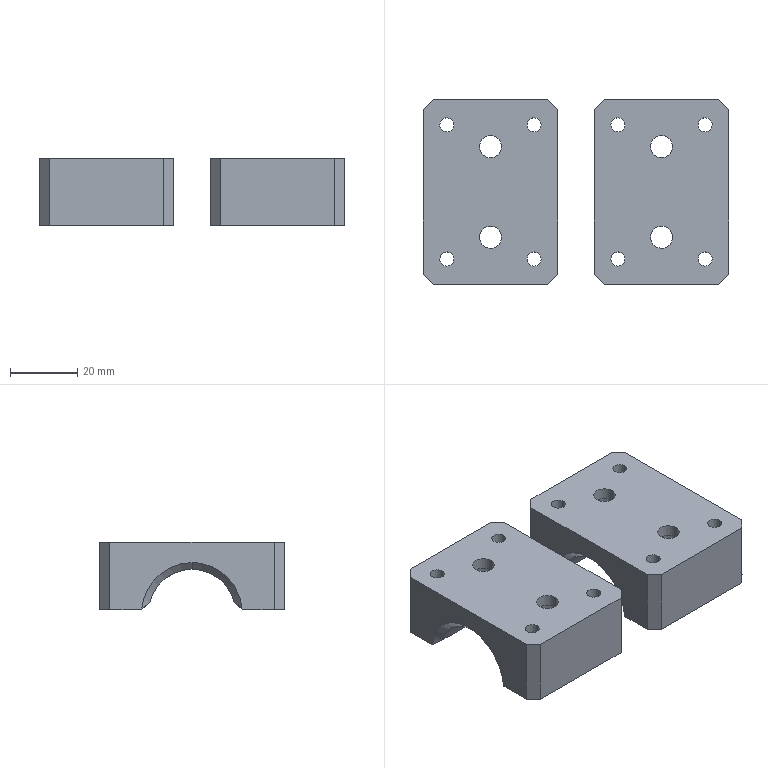NC program | NX | posted with a generic post | part box 91 x 55 x 20 mm
Lines 73 to 960 of 95737:
(ZLEVEL_PROFILE , TOOL : D10)
N126 T15 M6
N128 G54
N130 G17 G0 G90 X7.101 Y32.384 S9500 M3
N132 G43 Z30. H15
N134 Z1.5
N136 G94 G1 X7.946 Y32.6 Z1.454 F1000.
N138 X43.054 Z-0.386
N140 X44.463 Y32.24 Z-0.462
N142 X45.715 Y31.498 Z-0.538
N144 X49.498 Y27.715 Z-0.819
N146 X50.24 Y26.463 Z-0.895
N148 X50.6 Y25.054 Z-0.971
N150 Y24.5 Z-1.
N152 Y-24.5 F2800.
N154 G2 X49.106 Y-28.106 R5.1
N156 G1 X46.106 Y-31.106
N158 G2 X42.5 Y-32.6 R5.1
N160 G1 X8.5
N162 G2 X4.894 Y-31.106 R5.1
N164 G1 X1.894 Y-28.106
N166 G2 X0.4 Y-24.5 R5.1
N168 G1 Y24.5
N170 G2 X1.894 Y28.106 R5.1
N172 G1 X4.894 Y31.106
N174 G2 X8.5 Y32.6 R5.1
N176 G1 X42.5
N178 G2 X46.106 Y31.106 R5.1
N180 G1 X49.106 Y28.106
N182 G2 X50.6 Y24.5 R5.1
N184 G1 Y-24.274 Z-1.851
N186 X50.597 Y-24.661 Z-1.858
N188 X50.571 Y-25.047 Z-1.865
N190 X50.515 Y-25.43 Z-1.872
N192 X50.43 Y-25.808 Z-1.878
N194 X50.316 Y-26.178 Z-1.885
N196 X50.175 Y-26.538 Z-1.892
N198 X50.007 Y-26.887 Z-1.899
N200 X49.813 Y-27.221 Z-1.905
N202 X49.594 Y-27.541 Z-1.912
N204 X49.352 Y-27.842 Z-1.919
N206 X49.088 Y-28.125 Z-1.926
N208 X48.814 Y-28.399 Z-1.932
N210 X46.35 Y-30.862 Z-1.993
N212 X46.077 Y-31.136 Z-2.
N214 G2 X42.5 Y-32.6 R5.1
N216 G1 X8.5
N218 G2 X4.894 Y-31.106 R5.1
N220 G1 X1.894 Y-28.106
N222 G2 X0.4 Y-24.5 R5.1
N224 G1 Y24.5
N226 G2 X1.894 Y28.106 R5.1
N228 G1 X4.894 Y31.106
N230 G2 X8.5 Y32.6 R5.1
N232 G1 X42.5
N234 G2 X46.106 Y31.106 R5.1
N236 G1 X49.106 Y28.106
N238 G2 X50.6 Y24.5 R5.1
N240 G1 Y-24.274 Z-2.851
N242 X50.597 Y-24.661 Z-2.858
N244 X50.571 Y-25.047 Z-2.865
N246 X50.515 Y-25.43 Z-2.872
N248 X50.43 Y-25.808 Z-2.878
N250 X50.316 Y-26.178 Z-2.885
N252 X50.175 Y-26.538 Z-2.892
N254 X50.007 Y-26.887 Z-2.899
N256 X49.813 Y-27.221 Z-2.905
N258 X49.594 Y-27.541 Z-2.912
N260 X49.352 Y-27.842 Z-2.919
N262 X49.088 Y-28.125 Z-2.926
N264 X48.814 Y-28.399 Z-2.932
N266 X46.35 Y-30.862 Z-2.993
N268 X46.077 Y-31.136 Z-3.
N270 G2 X42.5 Y-32.6 R5.1
N272 G1 X8.5
N274 G2 X4.894 Y-31.106 R5.1
N276 G1 X1.894 Y-28.106
N278 G2 X0.4 Y-24.5 R5.1
N280 G1 Y24.5
N282 G2 X1.894 Y28.106 R5.1
N284 G1 X4.894 Y31.106
N286 G2 X8.5 Y32.6 R5.1
N288 G1 X42.5
N290 G2 X46.106 Y31.106 R5.1
N292 G1 X49.106 Y28.106
N294 G2 X50.6 Y24.5 R5.1
N296 G1 Y-24.274 Z-3.851
N298 X50.597 Y-24.661 Z-3.858
N300 X50.571 Y-25.047 Z-3.865
N302 X50.515 Y-25.43 Z-3.872
N304 X50.43 Y-25.808 Z-3.878
N306 X50.316 Y-26.178 Z-3.885
N308 X50.175 Y-26.538 Z-3.892
N310 X50.007 Y-26.887 Z-3.899
N312 X49.813 Y-27.221 Z-3.905
N314 X49.594 Y-27.541 Z-3.912
N316 X49.352 Y-27.842 Z-3.919
N318 X49.088 Y-28.125 Z-3.926
N320 X48.814 Y-28.399 Z-3.932
N322 X46.35 Y-30.862 Z-3.993
N324 X46.077 Y-31.136 Z-4.
N326 G2 X42.5 Y-32.6 R5.1
N328 G1 X8.5
N330 G2 X4.894 Y-31.106 R5.1
N332 G1 X1.894 Y-28.106
N334 G2 X0.4 Y-24.5 R5.1
N336 G1 Y24.5
N338 G2 X1.894 Y28.106 R5.1
N340 G1 X4.894 Y31.106
N342 G2 X8.5 Y32.6 R5.1
N344 G1 X42.5
N346 G2 X46.106 Y31.106 R5.1
N348 G1 X49.106 Y28.106
N350 G2 X50.6 Y24.5 R5.1
N352 G1 Y-24.274 Z-4.851
N354 X50.597 Y-24.661 Z-4.858
N356 X50.571 Y-25.047 Z-4.865
N358 X50.515 Y-25.43 Z-4.872
N360 X50.43 Y-25.808 Z-4.878
N362 X50.316 Y-26.178 Z-4.885
N364 X50.175 Y-26.538 Z-4.892
N366 X50.007 Y-26.887 Z-4.899
N368 X49.813 Y-27.221 Z-4.905
N370 X49.594 Y-27.541 Z-4.912
N372 X49.352 Y-27.842 Z-4.919
N374 X49.088 Y-28.125 Z-4.926
N376 X48.814 Y-28.399 Z-4.932
N378 X46.35 Y-30.862 Z-4.993
N380 X46.077 Y-31.136 Z-5.
N382 G2 X42.5 Y-32.6 R5.1
N384 G1 X8.5
N386 G2 X4.894 Y-31.106 R5.1
N388 G1 X1.894 Y-28.106
N390 G2 X0.4 Y-24.5 R5.1
N392 G1 Y24.5
N394 G2 X1.894 Y28.106 R5.1
N396 G1 X4.894 Y31.106
N398 G2 X8.5 Y32.6 R5.1
N400 G1 X42.5
N402 G2 X46.106 Y31.106 R5.1
N404 G1 X49.106 Y28.106
N406 G2 X50.6 Y24.5 R5.1
N408 G1 Y-24.274 Z-5.851
N410 X50.597 Y-24.661 Z-5.858
N412 X50.571 Y-25.047 Z-5.865
N414 X50.515 Y-25.43 Z-5.872
N416 X50.43 Y-25.808 Z-5.878
N418 X50.316 Y-26.178 Z-5.885
N420 X50.175 Y-26.538 Z-5.892
N422 X50.007 Y-26.887 Z-5.899
N424 X49.813 Y-27.221 Z-5.905
N426 X49.594 Y-27.541 Z-5.912
N428 X49.352 Y-27.842 Z-5.919
N430 X49.088 Y-28.125 Z-5.926
N432 X48.814 Y-28.399 Z-5.932
N434 X46.35 Y-30.862 Z-5.993
N436 X46.077 Y-31.136 Z-6.
N438 G2 X42.5 Y-32.6 R5.1
N440 G1 X8.5
N442 G2 X4.894 Y-31.106 R5.1
N444 G1 X1.894 Y-28.106
N446 G2 X0.4 Y-24.5 R5.1
N448 G1 Y24.5
N450 G2 X1.894 Y28.106 R5.1
N452 G1 X4.894 Y31.106
N454 G2 X8.5 Y32.6 R5.1
N456 G1 X42.5
N458 G2 X46.106 Y31.106 R5.1
N460 G1 X49.106 Y28.106
N462 G2 X50.6 Y24.5 R5.1
N464 G1 Y-24.274 Z-6.851
N466 X50.597 Y-24.661 Z-6.858
N468 X50.571 Y-25.047 Z-6.865
N470 X50.515 Y-25.43 Z-6.872
N472 X50.43 Y-25.808 Z-6.878
N474 X50.316 Y-26.178 Z-6.885
N476 X50.175 Y-26.538 Z-6.892
N478 X50.007 Y-26.887 Z-6.899
N480 X49.813 Y-27.221 Z-6.905
N482 X49.594 Y-27.541 Z-6.912
N484 X49.352 Y-27.842 Z-6.919
N486 X49.088 Y-28.125 Z-6.926
N488 X48.814 Y-28.399 Z-6.932
N490 X46.35 Y-30.862 Z-6.993
N492 X46.077 Y-31.136 Z-7.
N494 G2 X42.5 Y-32.6 R5.1
N496 G1 X8.5
N498 G2 X4.894 Y-31.106 R5.1
N500 G1 X1.894 Y-28.106
N502 G2 X0.4 Y-24.5 R5.1
N504 G1 Y24.5
N506 G2 X1.894 Y28.106 R5.1
N508 G1 X4.894 Y31.106
N510 G2 X8.5 Y32.6 R5.1
N512 G1 X42.5
N514 G2 X46.106 Y31.106 R5.1
N516 G1 X49.106 Y28.106
N518 G2 X50.6 Y24.5 R5.1
N520 G1 Y-24.274 Z-7.851
N522 X50.597 Y-24.661 Z-7.858
N524 X50.571 Y-25.047 Z-7.865
N526 X50.515 Y-25.43 Z-7.872
N528 X50.43 Y-25.808 Z-7.878
N530 X50.316 Y-26.178 Z-7.885
N532 X50.175 Y-26.538 Z-7.892
N534 X50.007 Y-26.887 Z-7.899
N536 X49.813 Y-27.221 Z-7.905
N538 X49.594 Y-27.541 Z-7.912
N540 X49.352 Y-27.842 Z-7.919
N542 X49.088 Y-28.125 Z-7.926
N544 X48.814 Y-28.399 Z-7.932
N546 X46.35 Y-30.862 Z-7.993
N548 X46.077 Y-31.136 Z-8.
N550 G2 X42.5 Y-32.6 R5.1
N552 G1 X8.5
N554 G2 X4.894 Y-31.106 R5.1
N556 G1 X1.894 Y-28.106
N558 G2 X0.4 Y-24.5 R5.1
N560 G1 Y24.5
N562 G2 X1.894 Y28.106 R5.1
N564 G1 X4.894 Y31.106
N566 G2 X8.5 Y32.6 R5.1
N568 G1 X42.5
N570 G2 X46.106 Y31.106 R5.1
N572 G1 X49.106 Y28.106
N574 G2 X50.6 Y24.5 R5.1
N576 G1 Y-24.274 Z-8.851
N578 X50.597 Y-24.661 Z-8.858
N580 X50.571 Y-25.047 Z-8.865
N582 X50.515 Y-25.43 Z-8.872
N584 X50.43 Y-25.808 Z-8.878
N586 X50.316 Y-26.178 Z-8.885
N588 X50.175 Y-26.538 Z-8.892
N590 X50.007 Y-26.887 Z-8.899
N592 X49.813 Y-27.221 Z-8.905
N594 X49.594 Y-27.541 Z-8.912
N596 X49.352 Y-27.842 Z-8.919
N598 X49.088 Y-28.125 Z-8.926
N600 X48.814 Y-28.399 Z-8.932
N602 X46.35 Y-30.862 Z-8.993
N604 X46.077 Y-31.136 Z-9.
N606 G2 X42.5 Y-32.6 R5.1
N608 G1 X8.5
N610 G2 X4.894 Y-31.106 R5.1
N612 G1 X1.894 Y-28.106
N614 G2 X0.4 Y-24.5 R5.1
N616 G1 Y24.5
N618 G2 X1.894 Y28.106 R5.1
N620 G1 X4.894 Y31.106
N622 G2 X8.5 Y32.6 R5.1
N624 G1 X42.5
N626 G2 X46.106 Y31.106 R5.1
N628 G1 X49.106 Y28.106
N630 G2 X50.6 Y24.5 R5.1
N632 G1 Y-24.274 Z-9.851
N634 X50.597 Y-24.661 Z-9.858
N636 X50.571 Y-25.047 Z-9.865
N638 X50.515 Y-25.43 Z-9.872
N640 X50.43 Y-25.808 Z-9.878
N642 X50.316 Y-26.178 Z-9.885
N644 X50.175 Y-26.538 Z-9.892
N646 X50.007 Y-26.887 Z-9.899
N648 X49.813 Y-27.221 Z-9.905
N650 X49.594 Y-27.541 Z-9.912
N652 X49.352 Y-27.842 Z-9.919
N654 X49.088 Y-28.125 Z-9.926
N656 X48.814 Y-28.399 Z-9.932
N658 X46.35 Y-30.862 Z-9.993
N660 X46.077 Y-31.136 Z-10.
N662 G2 X42.5 Y-32.6 R5.1
N664 G1 X8.5
N666 G2 X4.894 Y-31.106 R5.1
N668 G1 X1.894 Y-28.106
N670 G2 X0.4 Y-24.5 R5.1
N672 G1 Y24.5
N674 G2 X1.894 Y28.106 R5.1
N676 G1 X4.894 Y31.106
N678 G2 X8.5 Y32.6 R5.1
N680 G1 X42.5
N682 G2 X46.106 Y31.106 R5.1
N684 G1 X49.106 Y28.106
N686 G2 X50.6 Y24.5 R5.1
N688 G1 Y-24.274 Z-10.851
N690 X50.597 Y-24.661 Z-10.858
N692 X50.571 Y-25.047 Z-10.865
N694 X50.515 Y-25.43 Z-10.872
N696 X50.43 Y-25.808 Z-10.878
N698 X50.316 Y-26.178 Z-10.885
N700 X50.175 Y-26.538 Z-10.892
N702 X50.007 Y-26.887 Z-10.899
N704 X49.813 Y-27.221 Z-10.905
N706 X49.594 Y-27.541 Z-10.912
N708 X49.352 Y-27.842 Z-10.919
N710 X49.088 Y-28.125 Z-10.926
N712 X48.814 Y-28.399 Z-10.932
N714 X46.35 Y-30.862 Z-10.993
N716 X46.077 Y-31.136 Z-11.
N718 G2 X42.5 Y-32.6 R5.1
N720 G1 X8.5
N722 G2 X4.894 Y-31.106 R5.1
N724 G1 X1.894 Y-28.106
N726 G2 X0.4 Y-24.5 R5.1
N728 G1 Y24.5
N730 G2 X1.894 Y28.106 R5.1
N732 G1 X4.894 Y31.106
N734 G2 X8.5 Y32.6 R5.1
N736 G1 X42.5
N738 G2 X46.106 Y31.106 R5.1
N740 G1 X49.106 Y28.106
N742 G2 X50.6 Y24.5 R5.1
N744 G1 Y-24.274 Z-11.851
N746 X50.597 Y-24.661 Z-11.858
N748 X50.571 Y-25.047 Z-11.865
N750 X50.515 Y-25.43 Z-11.872
N752 X50.43 Y-25.808 Z-11.878
N754 X50.316 Y-26.178 Z-11.885
N756 X50.175 Y-26.538 Z-11.892
N758 X50.007 Y-26.887 Z-11.899
N760 X49.813 Y-27.221 Z-11.905
N762 X49.594 Y-27.541 Z-11.912
N764 X49.352 Y-27.842 Z-11.919
N766 X49.088 Y-28.125 Z-11.926
N768 X48.814 Y-28.399 Z-11.932
N770 X46.35 Y-30.862 Z-11.993
N772 X46.077 Y-31.136 Z-12.
N774 G2 X42.5 Y-32.6 R5.1
N776 G1 X8.5
N778 G2 X4.894 Y-31.106 R5.1
N780 G1 X1.894 Y-28.106
N782 G2 X0.4 Y-24.5 R5.1
N784 G1 Y24.5
N786 G2 X1.894 Y28.106 R5.1
N788 G1 X4.894 Y31.106
N790 G2 X8.5 Y32.6 R5.1
N792 G1 X42.5
N794 G2 X46.106 Y31.106 R5.1
N796 G1 X49.106 Y28.106
N798 G2 X50.6 Y24.5 R5.1
N800 G1 Y-24.274 Z-12.851
N802 X50.597 Y-24.661 Z-12.858
N804 X50.571 Y-25.047 Z-12.865
N806 X50.515 Y-25.43 Z-12.872
N808 X50.43 Y-25.808 Z-12.878
N810 X50.316 Y-26.178 Z-12.885
N812 X50.175 Y-26.538 Z-12.892
N814 X50.007 Y-26.887 Z-12.899
N816 X49.813 Y-27.221 Z-12.905
N818 X49.594 Y-27.541 Z-12.912
N820 X49.352 Y-27.842 Z-12.919
N822 X49.088 Y-28.125 Z-12.926
N824 X48.814 Y-28.399 Z-12.932
N826 X46.35 Y-30.862 Z-12.993
N828 X46.077 Y-31.136 Z-13.
N830 G2 X42.5 Y-32.6 R5.1
N832 G1 X8.5
N834 G2 X4.894 Y-31.106 R5.1
N836 G1 X1.894 Y-28.106
N838 G2 X0.4 Y-24.5 R5.1
N840 G1 Y24.5
N842 G2 X1.894 Y28.106 R5.1
N844 G1 X4.894 Y31.106
N846 G2 X8.5 Y32.6 R5.1
N848 G1 X42.5
N850 G2 X46.106 Y31.106 R5.1
N852 G1 X49.106 Y28.106
N854 G2 X50.6 Y24.5 R5.1
N856 G1 Y-24.274 Z-13.851
N858 X50.597 Y-24.661 Z-13.858
N860 X50.571 Y-25.047 Z-13.865
N862 X50.515 Y-25.43 Z-13.872
N864 X50.43 Y-25.808 Z-13.878
N866 X50.316 Y-26.178 Z-13.885
N868 X50.175 Y-26.538 Z-13.892
N870 X50.007 Y-26.887 Z-13.899
N872 X49.813 Y-27.221 Z-13.905
N874 X49.594 Y-27.541 Z-13.912
N876 X49.352 Y-27.842 Z-13.919
N878 X49.088 Y-28.125 Z-13.926
N880 X48.814 Y-28.399 Z-13.932
N882 X46.35 Y-30.862 Z-13.993
N884 X46.077 Y-31.136 Z-14.
N886 G2 X42.5 Y-32.6 R5.1
N888 G1 X8.5
N890 G2 X4.894 Y-31.106 R5.1
N892 G1 X1.894 Y-28.106
N894 G2 X0.4 Y-24.5 R5.1
N896 G1 Y24.5
N898 G2 X1.894 Y28.106 R5.1
N900 G1 X4.894 Y31.106
N902 G2 X8.5 Y32.6 R5.1
N904 G1 X42.5
N906 G2 X46.106 Y31.106 R5.1
N908 G1 X49.106 Y28.106
N910 G2 X50.6 Y24.5 R5.1
N912 G1 Y-24.274 Z-14.851
N914 X50.597 Y-24.661 Z-14.858
N916 X50.571 Y-25.047 Z-14.865
N918 X50.515 Y-25.43 Z-14.872
N920 X50.43 Y-25.808 Z-14.878
N922 X50.316 Y-26.178 Z-14.885
N924 X50.175 Y-26.538 Z-14.892
N926 X50.007 Y-26.887 Z-14.899
N928 X49.813 Y-27.221 Z-14.905
N930 X49.594 Y-27.541 Z-14.912
N932 X49.352 Y-27.842 Z-14.919
N934 X49.088 Y-28.125 Z-14.926
N936 X48.814 Y-28.399 Z-14.932
N938 X46.35 Y-30.862 Z-14.993
N940 X46.077 Y-31.136 Z-15.
N942 G2 X42.5 Y-32.6 R5.1
N944 G1 X8.5
N946 G2 X4.894 Y-31.106 R5.1
N948 G1 X1.894 Y-28.106
N950 G2 X0.4 Y-24.5 R5.1
N952 G1 Y24.5
N954 G2 X1.894 Y28.106 R5.1
N956 G1 X4.894 Y31.106
N958 G2 X8.5 Y32.6 R5.1
N960 G1 X42.5
N962 G2 X46.106 Y31.106 R5.1
N964 G1 X49.106 Y28.106
N966 G2 X50.6 Y24.5 R5.1
N968 G1 Y-24.274 Z-15.851
N970 X50.597 Y-24.661 Z-15.858
N972 X50.571 Y-25.047 Z-15.865
N974 X50.515 Y-25.43 Z-15.872
N976 X50.43 Y-25.808 Z-15.878
N978 X50.316 Y-26.178 Z-15.885
N980 X50.175 Y-26.538 Z-15.892
N982 X50.007 Y-26.887 Z-15.899
N984 X49.813 Y-27.221 Z-15.905
N986 X49.594 Y-27.541 Z-15.912
N988 X49.352 Y-27.842 Z-15.919
N990 X49.088 Y-28.125 Z-15.926
N992 X48.814 Y-28.399 Z-15.932
N994 X46.35 Y-30.862 Z-15.993
N996 X46.077 Y-31.136 Z-16.
N998 G2 X42.5 Y-32.6 R5.1
N1000 G1 X8.5
N1002 G2 X4.894 Y-31.106 R5.1
N1004 G1 X1.894 Y-28.106
N1006 G2 X0.4 Y-24.5 R5.1
N1008 G1 Y24.5
N1010 G2 X1.894 Y28.106 R5.1
N1012 G1 X4.894 Y31.106
N1014 G2 X8.5 Y32.6 R5.1
N1016 G1 X42.5
N1018 G2 X46.106 Y31.106 R5.1
N1020 G1 X49.106 Y28.106
N1022 G2 X50.6 Y24.5 R5.1
N1024 G1 Y-24.274 Z-16.851
N1026 X50.597 Y-24.661 Z-16.858
N1028 X50.571 Y-25.047 Z-16.865
N1030 X50.515 Y-25.43 Z-16.872
N1032 X50.43 Y-25.808 Z-16.878
N1034 X50.316 Y-26.178 Z-16.885
N1036 X50.175 Y-26.538 Z-16.892
N1038 X50.007 Y-26.887 Z-16.899
N1040 X49.813 Y-27.221 Z-16.905
N1042 X49.594 Y-27.541 Z-16.912
N1044 X49.352 Y-27.842 Z-16.919
N1046 X49.088 Y-28.125 Z-16.926
N1048 X48.814 Y-28.399 Z-16.932
N1050 X46.35 Y-30.862 Z-16.993
N1052 X46.077 Y-31.136 Z-17.
N1054 G2 X42.5 Y-32.6 R5.1
N1056 G1 X8.5
N1058 G2 X4.894 Y-31.106 R5.1
N1060 G1 X1.894 Y-28.106
N1062 G2 X0.4 Y-24.5 R5.1
N1064 G1 Y24.5
N1066 G2 X1.894 Y28.106 R5.1
N1068 G1 X4.894 Y31.106
N1070 G2 X8.5 Y32.6 R5.1
N1072 G1 X42.5
N1074 G2 X46.106 Y31.106 R5.1
N1076 G1 X49.106 Y28.106
N1078 G2 X50.6 Y24.5 R5.1
N1080 G1 Y-24.274 Z-17.851
N1082 X50.597 Y-24.661 Z-17.858
N1084 X50.571 Y-25.047 Z-17.865
N1086 X50.515 Y-25.43 Z-17.872
N1088 X50.43 Y-25.808 Z-17.878
N1090 X50.316 Y-26.178 Z-17.885
N1092 X50.175 Y-26.538 Z-17.892
N1094 X50.007 Y-26.887 Z-17.899
N1096 X49.813 Y-27.221 Z-17.905
N1098 X49.594 Y-27.541 Z-17.912
N1100 X49.352 Y-27.842 Z-17.919
N1102 X49.088 Y-28.125 Z-17.926
N1104 X48.814 Y-28.399 Z-17.932
N1106 X46.35 Y-30.862 Z-17.993
N1108 X46.077 Y-31.136 Z-18.
N1110 G2 X42.5 Y-32.6 R5.1
N1112 G1 X8.5
N1114 G2 X4.894 Y-31.106 R5.1
N1116 G1 X1.894 Y-28.106
N1118 G2 X0.4 Y-24.5 R5.1
N1120 G1 Y24.5
N1122 G2 X1.894 Y28.106 R5.1
N1124 G1 X4.894 Y31.106
N1126 G2 X8.5 Y32.6 R5.1
N1128 G1 X42.5
N1130 G2 X46.106 Y31.106 R5.1
N1132 G1 X49.106 Y28.106
N1134 G2 X50.6 Y24.5 R5.1
N1136 G1 Y-24.274 Z-18.851
N1138 X50.597 Y-24.661 Z-18.858
N1140 X50.571 Y-25.047 Z-18.865
N1142 X50.515 Y-25.43 Z-18.872
N1144 X50.43 Y-25.808 Z-18.878
N1146 X50.316 Y-26.178 Z-18.885
N1148 X50.175 Y-26.538 Z-18.892
N1150 X50.007 Y-26.887 Z-18.899
N1152 X49.813 Y-27.221 Z-18.905
N1154 X49.594 Y-27.541 Z-18.912
N1156 X49.352 Y-27.842 Z-18.919
N1158 X49.088 Y-28.125 Z-18.926
N1160 X48.814 Y-28.399 Z-18.932
N1162 X46.35 Y-30.862 Z-18.993
N1164 X46.077 Y-31.136 Z-19.
N1166 G2 X42.5 Y-32.6 R5.1
N1168 G1 X8.5
N1170 G2 X4.894 Y-31.106 R5.1
N1172 G1 X1.894 Y-28.106
N1174 G2 X0.4 Y-24.5 R5.1
N1176 G1 Y24.5
N1178 G2 X1.894 Y28.106 R5.1
N1180 G1 X4.894 Y31.106
N1182 G2 X8.5 Y32.6 R5.1
N1184 G1 X42.5
N1186 G2 X46.106 Y31.106 R5.1
N1188 G1 X49.106 Y28.106
N1190 G2 X50.6 Y24.5 R5.1
N1192 G1 Y-24.274 Z-19.851
N1194 X50.597 Y-24.661 Z-19.858
N1196 X50.571 Y-25.047 Z-19.865
N1198 X50.515 Y-25.43 Z-19.872
N1200 X50.43 Y-25.808 Z-19.878
N1202 X50.316 Y-26.178 Z-19.885
N1204 X50.175 Y-26.538 Z-19.892
N1206 X50.007 Y-26.887 Z-19.899
N1208 X49.813 Y-27.221 Z-19.905
N1210 X49.594 Y-27.541 Z-19.912
N1212 X49.352 Y-27.842 Z-19.919
N1214 X49.088 Y-28.125 Z-19.926
N1216 X48.814 Y-28.399 Z-19.932
N1218 X46.35 Y-30.862 Z-19.993
N1220 X46.077 Y-31.136 Z-20.
N1222 G2 X42.5 Y-32.6 R5.1
N1224 G1 X8.5
N1226 G2 X4.894 Y-31.106 R5.1
N1228 G1 X1.894 Y-28.106
N1230 G2 X0.4 Y-24.5 R5.1
N1232 G1 Y24.5
N1234 G2 X1.894 Y28.106 R5.1
N1236 G1 X4.894 Y31.106
N1238 G2 X8.5 Y32.6 R5.1
N1240 G1 X42.5
N1242 G2 X46.106 Y31.106 R5.1
N1244 G1 X49.106 Y28.106
N1246 G2 X50.6 Y24.5 R5.1
N1248 G1 Y-24.5
N1250 G2 X49.106 Y-28.106 R5.1
N1252 G1 X46.077 Y-31.136
N1254 Z-18.5
N1256 G0 Z53.
N1258 X-7.101 Y-32.384
N1260 Z1.5
N1262 G1 X-7.946 Y-32.6 Z1.454 F1000.
N1264 X-43.054 Z-0.386
N1266 X-44.463 Y-32.24 Z-0.462
N1268 X-45.715 Y-31.498 Z-0.538
N1270 X-49.498 Y-27.715 Z-0.819
N1272 X-50.24 Y-26.463 Z-0.895
N1274 X-50.6 Y-25.054 Z-0.971
N1276 Y-24.5 Z-1.
N1278 Y24.5 F2800.
N1280 G2 X-49.106 Y28.106 R5.1
N1282 G1 X-46.106 Y31.106
N1284 G2 X-42.5 Y32.6 R5.1
N1286 G1 X-8.5
N1288 G2 X-4.894 Y31.106 R5.1
N1290 G1 X-1.894 Y28.106
N1292 G2 X-0.4 Y24.5 R5.1
N1294 G1 Y-24.5
N1296 G2 X-1.894 Y-28.106 R5.1
N1298 G1 X-4.894 Y-31.106
N1300 G2 X-8.5 Y-32.6 R5.1
N1302 G1 X-42.5
N1304 G2 X-46.106 Y-31.106 R5.1
N1306 G1 X-49.106 Y-28.106
N1308 G2 X-50.6 Y-24.5 R5.1
N1310 G1 Y24.274 Z-1.851
N1312 X-50.597 Y24.661 Z-1.858
N1314 X-50.571 Y25.047 Z-1.865
N1316 X-50.515 Y25.43 Z-1.872
N1318 X-50.43 Y25.808 Z-1.878
N1320 X-50.316 Y26.178 Z-1.885
N1322 X-50.175 Y26.538 Z-1.892
N1324 X-50.007 Y26.887 Z-1.899
N1326 X-49.813 Y27.221 Z-1.905
N1328 X-49.594 Y27.541 Z-1.912
N1330 X-49.352 Y27.842 Z-1.919
N1332 X-49.088 Y28.125 Z-1.926
N1334 X-48.814 Y28.399 Z-1.932
N1336 X-46.35 Y30.862 Z-1.993
N1338 X-46.077 Y31.136 Z-2.
N1340 G2 X-42.5 Y32.6 R5.1
N1342 G1 X-8.5
N1344 G2 X-4.894 Y31.106 R5.1
N1346 G1 X-1.894 Y28.106
N1348 G2 X-0.4 Y24.5 R5.1
N1350 G1 Y-24.5
N1352 G2 X-1.894 Y-28.106 R5.1
N1354 G1 X-4.894 Y-31.106
N1356 G2 X-8.5 Y-32.6 R5.1
N1358 G1 X-42.5
N1360 G2 X-46.106 Y-31.106 R5.1
N1362 G1 X-49.106 Y-28.106
N1364 G2 X-50.6 Y-24.5 R5.1
N1366 G1 Y24.274 Z-2.851
N1368 X-50.597 Y24.661 Z-2.858
N1370 X-50.571 Y25.047 Z-2.865
N1372 X-50.515 Y25.43 Z-2.872
N1374 X-50.43 Y25.808 Z-2.878
N1376 X-50.316 Y26.178 Z-2.885
N1378 X-50.175 Y26.538 Z-2.892
N1380 X-50.007 Y26.887 Z-2.899
N1382 X-49.813 Y27.221 Z-2.905
N1384 X-49.594 Y27.541 Z-2.912
N1386 X-49.352 Y27.842 Z-2.919
N1388 X-49.088 Y28.125 Z-2.926
N1390 X-48.814 Y28.399 Z-2.932
N1392 X-46.35 Y30.862 Z-2.993
N1394 X-46.077 Y31.136 Z-3.
N1396 G2 X-42.5 Y32.6 R5.1
N1398 G1 X-8.5
N1400 G2 X-4.894 Y31.106 R5.1
N1402 G1 X-1.894 Y28.106
N1404 G2 X-0.4 Y24.5 R5.1
N1406 G1 Y-24.5
N1408 G2 X-1.894 Y-28.106 R5.1
N1410 G1 X-4.894 Y-31.106
N1412 G2 X-8.5 Y-32.6 R5.1
N1414 G1 X-42.5
N1416 G2 X-46.106 Y-31.106 R5.1
N1418 G1 X-49.106 Y-28.106
N1420 G2 X-50.6 Y-24.5 R5.1
N1422 G1 Y24.274 Z-3.851
N1424 X-50.597 Y24.661 Z-3.858
N1426 X-50.571 Y25.047 Z-3.865
N1428 X-50.515 Y25.43 Z-3.872
N1430 X-50.43 Y25.808 Z-3.878
N1432 X-50.316 Y26.178 Z-3.885
N1434 X-50.175 Y26.538 Z-3.892
N1436 X-50.007 Y26.887 Z-3.899
N1438 X-49.813 Y27.221 Z-3.905
N1440 X-49.594 Y27.541 Z-3.912
N1442 X-49.352 Y27.842 Z-3.919
N1444 X-49.088 Y28.125 Z-3.926
N1446 X-48.814 Y28.399 Z-3.932
N1448 X-46.35 Y30.862 Z-3.993
N1450 X-46.077 Y31.136 Z-4.
N1452 G2 X-42.5 Y32.6 R5.1
N1454 G1 X-8.5
N1456 G2 X-4.894 Y31.106 R5.1
N1458 G1 X-1.894 Y28.106
N1460 G2 X-0.4 Y24.5 R5.1
N1462 G1 Y-24.5
N1464 G2 X-1.894 Y-28.106 R5.1
N1466 G1 X-4.894 Y-31.106
N1468 G2 X-8.5 Y-32.6 R5.1
N1470 G1 X-42.5
N1472 G2 X-46.106 Y-31.106 R5.1
N1474 G1 X-49.106 Y-28.106
N1476 G2 X-50.6 Y-24.5 R5.1
N1478 G1 Y24.274 Z-4.851
N1480 X-50.597 Y24.661 Z-4.858
N1482 X-50.571 Y25.047 Z-4.865
N1484 X-50.515 Y25.43 Z-4.872
N1486 X-50.43 Y25.808 Z-4.878
N1488 X-50.316 Y26.178 Z-4.885
N1490 X-50.175 Y26.538 Z-4.892
N1492 X-50.007 Y26.887 Z-4.899
N1494 X-49.813 Y27.221 Z-4.905
N1496 X-49.594 Y27.541 Z-4.912
N1498 X-49.352 Y27.842 Z-4.919
N1500 X-49.088 Y28.125 Z-4.926
N1502 X-48.814 Y28.399 Z-4.932
N1504 X-46.35 Y30.862 Z-4.993
N1506 X-46.077 Y31.136 Z-5.
N1508 G2 X-42.5 Y32.6 R5.1
N1510 G1 X-8.5
N1512 G2 X-4.894 Y31.106 R5.1
N1514 G1 X-1.894 Y28.106
N1516 G2 X-0.4 Y24.5 R5.1
N1518 G1 Y-24.5
N1520 G2 X-1.894 Y-28.106 R5.1
N1522 G1 X-4.894 Y-31.106
N1524 G2 X-8.5 Y-32.6 R5.1
N1526 G1 X-42.5
N1528 G2 X-46.106 Y-31.106 R5.1
N1530 G1 X-49.106 Y-28.106
N1532 G2 X-50.6 Y-24.5 R5.1
N1534 G1 Y24.274 Z-5.851
N1536 X-50.597 Y24.661 Z-5.858
N1538 X-50.571 Y25.047 Z-5.865
N1540 X-50.515 Y25.43 Z-5.872
N1542 X-50.43 Y25.808 Z-5.878
N1544 X-50.316 Y26.178 Z-5.885
N1546 X-50.175 Y26.538 Z-5.892
N1548 X-50.007 Y26.887 Z-5.899
N1550 X-49.813 Y27.221 Z-5.905
N1552 X-49.594 Y27.541 Z-5.912
N1554 X-49.352 Y27.842 Z-5.919
N1556 X-49.088 Y28.125 Z-5.926
N1558 X-48.814 Y28.399 Z-5.932
N1560 X-46.35 Y30.862 Z-5.993
N1562 X-46.077 Y31.136 Z-6.
N1564 G2 X-42.5 Y32.6 R5.1
N1566 G1 X-8.5
N1568 G2 X-4.894 Y31.106 R5.1
N1570 G1 X-1.894 Y28.106
N1572 G2 X-0.4 Y24.5 R5.1
N1574 G1 Y-24.5
N1576 G2 X-1.894 Y-28.106 R5.1
N1578 G1 X-4.894 Y-31.106
N1580 G2 X-8.5 Y-32.6 R5.1
N1582 G1 X-42.5
N1584 G2 X-46.106 Y-31.106 R5.1
N1586 G1 X-49.106 Y-28.106
N1588 G2 X-50.6 Y-24.5 R5.1
N1590 G1 Y24.274 Z-6.851
N1592 X-50.597 Y24.661 Z-6.858
N1594 X-50.571 Y25.047 Z-6.865
N1596 X-50.515 Y25.43 Z-6.872
N1598 X-50.43 Y25.808 Z-6.878
N1600 X-50.316 Y26.178 Z-6.885
N1602 X-50.175 Y26.538 Z-6.892
N1604 X-50.007 Y26.887 Z-6.899
N1606 X-49.813 Y27.221 Z-6.905
N1608 X-49.594 Y27.541 Z-6.912
N1610 X-49.352 Y27.842 Z-6.919
N1612 X-49.088 Y28.125 Z-6.926
N1614 X-48.814 Y28.399 Z-6.932
N1616 X-46.35 Y30.862 Z-6.993
N1618 X-46.077 Y31.136 Z-7.
N1620 G2 X-42.5 Y32.6 R5.1
N1622 G1 X-8.5
N1624 G2 X-4.894 Y31.106 R5.1
N1626 G1 X-1.894 Y28.106
N1628 G2 X-0.4 Y24.5 R5.1
N1630 G1 Y-24.5
N1632 G2 X-1.894 Y-28.106 R5.1
N1634 G1 X-4.894 Y-31.106
N1636 G2 X-8.5 Y-32.6 R5.1
N1638 G1 X-42.5
N1640 G2 X-46.106 Y-31.106 R5.1
N1642 G1 X-49.106 Y-28.106
N1644 G2 X-50.6 Y-24.5 R5.1
N1646 G1 Y24.274 Z-7.851
N1648 X-50.597 Y24.661 Z-7.858
N1650 X-50.571 Y25.047 Z-7.865
N1652 X-50.515 Y25.43 Z-7.872
N1654 X-50.43 Y25.808 Z-7.878
N1656 X-50.316 Y26.178 Z-7.885
N1658 X-50.175 Y26.538 Z-7.892
N1660 X-50.007 Y26.887 Z-7.899
N1662 X-49.813 Y27.221 Z-7.905
N1664 X-49.594 Y27.541 Z-7.912
N1666 X-49.352 Y27.842 Z-7.919
N1668 X-49.088 Y28.125 Z-7.926
N1670 X-48.814 Y28.399 Z-7.932
N1672 X-46.35 Y30.862 Z-7.993
N1674 X-46.077 Y31.136 Z-8.
N1676 G2 X-42.5 Y32.6 R5.1
N1678 G1 X-8.5
N1680 G2 X-4.894 Y31.106 R5.1
N1682 G1 X-1.894 Y28.106
N1684 G2 X-0.4 Y24.5 R5.1
N1686 G1 Y-24.5
N1688 G2 X-1.894 Y-28.106 R5.1
N1690 G1 X-4.894 Y-31.106
N1692 G2 X-8.5 Y-32.6 R5.1
N1694 G1 X-42.5
N1696 G2 X-46.106 Y-31.106 R5.1
N1698 G1 X-49.106 Y-28.106
N1700 G2 X-50.6 Y-24.5 R5.1
N1702 G1 Y24.274 Z-8.851
N1704 X-50.597 Y24.661 Z-8.858
N1706 X-50.571 Y25.047 Z-8.865
N1708 X-50.515 Y25.43 Z-8.872
N1710 X-50.43 Y25.808 Z-8.878
N1712 X-50.316 Y26.178 Z-8.885
N1714 X-50.175 Y26.538 Z-8.892
N1716 X-50.007 Y26.887 Z-8.899
N1718 X-49.813 Y27.221 Z-8.905
N1720 X-49.594 Y27.541 Z-8.912
N1722 X-49.352 Y27.842 Z-8.919
N1724 X-49.088 Y28.125 Z-8.926
N1726 X-48.814 Y28.399 Z-8.932
N1728 X-46.35 Y30.862 Z-8.993
N1730 X-46.077 Y31.136 Z-9.
N1732 G2 X-42.5 Y32.6 R5.1
N1734 G1 X-8.5
N1736 G2 X-4.894 Y31.106 R5.1
N1738 G1 X-1.894 Y28.106
N1740 G2 X-0.4 Y24.5 R5.1
N1742 G1 Y-24.5
N1744 G2 X-1.894 Y-28.106 R5.1
N1746 G1 X-4.894 Y-31.106
N1748 G2 X-8.5 Y-32.6 R5.1
N1750 G1 X-42.5
N1752 G2 X-46.106 Y-31.106 R5.1
N1754 G1 X-49.106 Y-28.106
N1756 G2 X-50.6 Y-24.5 R5.1
N1758 G1 Y24.274 Z-9.851
N1760 X-50.597 Y24.661 Z-9.858
N1762 X-50.571 Y25.047 Z-9.865
N1764 X-50.515 Y25.43 Z-9.872
N1766 X-50.43 Y25.808 Z-9.878
N1768 X-50.316 Y26.178 Z-9.885
N1770 X-50.175 Y26.538 Z-9.892
N1772 X-50.007 Y26.887 Z-9.899
N1774 X-49.813 Y27.221 Z-9.905
N1776 X-49.594 Y27.541 Z-9.912
N1778 X-49.352 Y27.842 Z-9.919
N1780 X-49.088 Y28.125 Z-9.926
N1782 X-48.814 Y28.399 Z-9.932
N1784 X-46.35 Y30.862 Z-9.993
N1786 X-46.077 Y31.136 Z-10.
N1788 G2 X-42.5 Y32.6 R5.1
N1790 G1 X-8.5
N1792 G2 X-4.894 Y31.106 R5.1
N1794 G1 X-1.894 Y28.106
N1796 G2 X-0.4 Y24.5 R5.1
N1798 G1 Y-24.5
N1800 G2 X-1.894 Y-28.106 R5.1
N1802 G1 X-4.894 Y-31.106
N1804 G2 X-8.5 Y-32.6 R5.1
N1806 G1 X-42.5
N1808 G2 X-46.106 Y-31.106 R5.1
N1810 G1 X-49.106 Y-28.106
N1812 G2 X-50.6 Y-24.5 R5.1
N1814 G1 Y24.274 Z-10.851
N1816 X-50.597 Y24.661 Z-10.858
N1818 X-50.571 Y25.047 Z-10.865
N1820 X-50.515 Y25.43 Z-10.872
N1822 X-50.43 Y25.808 Z-10.878
N1824 X-50.316 Y26.178 Z-10.885
N1826 X-50.175 Y26.538 Z-10.892
N1828 X-50.007 Y26.887 Z-10.899
N1830 X-49.813 Y27.221 Z-10.905
N1832 X-49.594 Y27.541 Z-10.912
N1834 X-49.352 Y27.842 Z-10.919
N1836 X-49.088 Y28.125 Z-10.926
N1838 X-48.814 Y28.399 Z-10.932
N1840 X-46.35 Y30.862 Z-10.993
N1842 X-46.077 Y31.136 Z-11.
N1844 G2 X-42.5 Y32.6 R5.1
N1846 G1 X-8.5
N1848 G2 X-4.894 Y31.106 R5.1
N1850 G1 X-1.894 Y28.106
N1852 G2 X-0.4 Y24.5 R5.1
N1854 G1 Y-24.5
N1856 G2 X-1.894 Y-28.106 R5.1
N1858 G1 X-4.894 Y-31.106
N1860 G2 X-8.5 Y-32.6 R5.1
N1862 G1 X-42.5
N1864 G2 X-46.106 Y-31.106 R5.1
N1866 G1 X-49.106 Y-28.106
N1868 G2 X-50.6 Y-24.5 R5.1
N1870 G1 Y24.274 Z-11.851
N1872 X-50.597 Y24.661 Z-11.858
N1874 X-50.571 Y25.047 Z-11.865
N1876 X-50.515 Y25.43 Z-11.872
N1878 X-50.43 Y25.808 Z-11.878
N1880 X-50.316 Y26.178 Z-11.885
N1882 X-50.175 Y26.538 Z-11.892
N1884 X-50.007 Y26.887 Z-11.899
N1886 X-49.813 Y27.221 Z-11.905
N1888 X-49.594 Y27.541 Z-11.912
N1890 X-49.352 Y27.842 Z-11.919
N1892 X-49.088 Y28.125 Z-11.926
N1894 X-48.814 Y28.399 Z-11.932